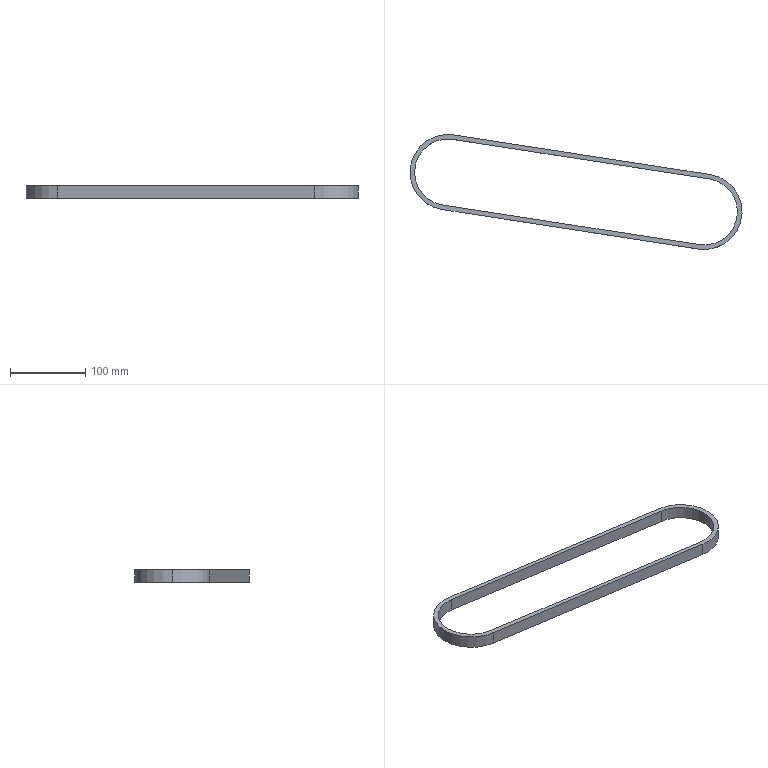Part | SolidWorks | features BeltProfileFeature 1, ExtruThin 1 | 1 solid | 12 faces | box 440 x 152.5 x 17 mm | volume 100304 mm3 | cylinder 6 | plane 6 | commonest cylinder face diameters 88 x3 100 x3
STEP:
#1=CARTESIAN_POINT('',(-44.,0.,8.5));
#2=VERTEX_POINT('',#1);
#3=CARTESIAN_POINT('',(6.715,43.485,8.5));
#4=VERTEX_POINT('',#3);
#5=CARTESIAN_POINT('',(0.,0.,8.5));
#6=DIRECTION('',(0.,0.,-1.));
#7=DIRECTION('',(-1.,0.,0.));
#8=AXIS2_PLACEMENT_3D('',#5,#6,#7);
#9=CIRCLE('',#8,44.);
#10=EDGE_CURVE('',#2,#4,#9,.T.);
#11=ORIENTED_EDGE('',*,*,#10,.F.);
#12=CARTESIAN_POINT('',(-44.,0.,-8.5));
#13=VERTEX_POINT('',#12);
#14=CARTESIAN_POINT('',(-44.,0.,8.5));
#15=DIRECTION('',(0.,0.,-1.));
#16=VECTOR('',#15,1000.);
#17=LINE('',#14,#16);
#18=EDGE_CURVE('',#2,#13,#17,.T.);
#19=ORIENTED_EDGE('',*,*,#18,.T.);
#20=CARTESIAN_POINT('',(6.715,43.485,-8.5));
#21=VERTEX_POINT('',#20);
#22=CARTESIAN_POINT('',(0.,0.,-8.5));
#23=DIRECTION('',(0.,0.,-1.));
#24=DIRECTION('',(-1.,0.,0.));
#25=AXIS2_PLACEMENT_3D('',#22,#23,#24);
#26=CIRCLE('',#25,44.);
#27=EDGE_CURVE('',#13,#21,#26,.T.);
#28=ORIENTED_EDGE('',*,*,#27,.T.);
#29=CARTESIAN_POINT('',(6.715,43.485,8.5));
#30=DIRECTION('',(0.,0.,-1.));
#31=VECTOR('',#30,1000.);
#32=LINE('',#29,#31);
#33=EDGE_CURVE('',#4,#21,#32,.T.);
#34=ORIENTED_EDGE('',*,*,#33,.F.);
#35=EDGE_LOOP('',(#11,#19,#28,#34));
#36=FACE_OUTER_BOUND('',#35,.T.);
#37=CARTESIAN_POINT('',(0.,0.,8.5));
#38=DIRECTION('',(0.,0.,-1.));
#39=DIRECTION('',(-1.,0.,0.));
#40=AXIS2_PLACEMENT_3D('',#37,#38,#39);
#41=CYLINDRICAL_SURFACE('',#40,44.);
#42=ADVANCED_FACE('',(#36),#41,.F.);
#43=CARTESIAN_POINT('',(-7.63,-49.414,8.5));
#44=VERTEX_POINT('',#43);
#45=CARTESIAN_POINT('',(-50.,0.,8.5));
#46=VERTEX_POINT('',#45);
#47=CARTESIAN_POINT('',(0.,0.,8.5));
#48=DIRECTION('',(0.,0.,-1.));
#49=DIRECTION('',(-1.,0.,0.));
#50=AXIS2_PLACEMENT_3D('',#47,#48,#49);
#51=CIRCLE('',#50,50.);
#52=EDGE_CURVE('',#44,#46,#51,.T.);
#53=ORIENTED_EDGE('',*,*,#52,.T.);
#54=CARTESIAN_POINT('',(-50.,0.,-8.5));
#55=VERTEX_POINT('',#54);
#56=CARTESIAN_POINT('',(-50.,0.,8.5));
#57=DIRECTION('',(0.,0.,-1.));
#58=VECTOR('',#57,1000.);
#59=LINE('',#56,#58);
#60=EDGE_CURVE('',#46,#55,#59,.T.);
#61=ORIENTED_EDGE('',*,*,#60,.T.);
#62=CARTESIAN_POINT('',(-7.63,-49.414,-8.5));
#63=VERTEX_POINT('',#62);
#64=CARTESIAN_POINT('',(0.,0.,-8.5));
#65=DIRECTION('',(0.,0.,-1.));
#66=DIRECTION('',(-1.,0.,0.));
#67=AXIS2_PLACEMENT_3D('',#64,#65,#66);
#68=CIRCLE('',#67,50.);
#69=EDGE_CURVE('',#63,#55,#68,.T.);
#70=ORIENTED_EDGE('',*,*,#69,.F.);
#71=CARTESIAN_POINT('',(-7.63,-49.414,8.5));
#72=DIRECTION('',(0.,0.,-1.));
#73=VECTOR('',#72,1000.);
#74=LINE('',#71,#73);
#75=EDGE_CURVE('',#44,#63,#74,.T.);
#76=ORIENTED_EDGE('',*,*,#75,.F.);
#77=EDGE_LOOP('',(#53,#61,#70,#76));
#78=FACE_OUTER_BOUND('',#77,.T.);
#79=CARTESIAN_POINT('',(0.,0.,8.5));
#80=DIRECTION('',(0.,0.,-1.));
#81=DIRECTION('',(-1.,0.,0.));
#82=AXIS2_PLACEMENT_3D('',#79,#80,#81);
#83=CYLINDRICAL_SURFACE('',#82,50.);
#84=ADVANCED_FACE('',(#78),#83,.T.);
#85=CARTESIAN_POINT('',(332.37,-101.914,-8.5));
#86=VERTEX_POINT('',#85);
#87=CARTESIAN_POINT('',(332.37,-101.914,-8.5));
#88=DIRECTION('',(-0.9883,0.1526,0.));
#89=VECTOR('',#88,1000.);
#90=LINE('',#87,#89);
#91=EDGE_CURVE('',#86,#63,#90,.T.);
#92=ORIENTED_EDGE('',*,*,#91,.F.);
#93=CARTESIAN_POINT('',(332.37,-101.914,8.5));
#94=VERTEX_POINT('',#93);
#95=CARTESIAN_POINT('',(332.37,-101.914,8.5));
#96=DIRECTION('',(0.,0.,-1.));
#97=VECTOR('',#96,1000.);
#98=LINE('',#95,#97);
#99=EDGE_CURVE('',#94,#86,#98,.T.);
#100=ORIENTED_EDGE('',*,*,#99,.F.);
#101=CARTESIAN_POINT('',(332.37,-101.914,8.5));
#102=DIRECTION('',(-0.9883,0.1526,0.));
#103=VECTOR('',#102,1000.);
#104=LINE('',#101,#103);
#105=EDGE_CURVE('',#94,#44,#104,.T.);
#106=ORIENTED_EDGE('',*,*,#105,.T.);
#107=ORIENTED_EDGE('',*,*,#75,.T.);
#108=EDGE_LOOP('',(#92,#100,#106,#107));
#109=FACE_OUTER_BOUND('',#108,.T.);
#110=CARTESIAN_POINT('',(332.37,-101.914,8.5));
#111=DIRECTION('',(-0.1526,-0.9883,0.));
#112=DIRECTION('',(0.9883,-0.1526,0.));
#113=AXIS2_PLACEMENT_3D('',#110,#111,#112);
#114=PLANE('',#113);
#115=ADVANCED_FACE('',(#109),#114,.T.);
#116=CARTESIAN_POINT('',(347.63,-3.086,-8.5));
#117=VERTEX_POINT('',#116);
#118=CARTESIAN_POINT('',(340.,-52.5,-8.5));
#119=DIRECTION('',(0.,0.,-1.));
#120=DIRECTION('',(-1.,0.,0.));
#121=AXIS2_PLACEMENT_3D('',#118,#119,#120);
#122=CIRCLE('',#121,50.);
#123=EDGE_CURVE('',#117,#86,#122,.T.);
#124=ORIENTED_EDGE('',*,*,#123,.F.);
#125=CARTESIAN_POINT('',(347.63,-3.086,8.5));
#126=VERTEX_POINT('',#125);
#127=CARTESIAN_POINT('',(347.63,-3.086,8.5));
#128=DIRECTION('',(0.,0.,-1.));
#129=VECTOR('',#128,1000.);
#130=LINE('',#127,#129);
#131=EDGE_CURVE('',#126,#117,#130,.T.);
#132=ORIENTED_EDGE('',*,*,#131,.F.);
#133=CARTESIAN_POINT('',(340.,-52.5,8.5));
#134=DIRECTION('',(0.,0.,-1.));
#135=DIRECTION('',(-1.,0.,0.));
#136=AXIS2_PLACEMENT_3D('',#133,#134,#135);
#137=CIRCLE('',#136,50.);
#138=EDGE_CURVE('',#126,#94,#137,.T.);
#139=ORIENTED_EDGE('',*,*,#138,.T.);
#140=ORIENTED_EDGE('',*,*,#99,.T.);
#141=EDGE_LOOP('',(#124,#132,#139,#140));
#142=FACE_OUTER_BOUND('',#141,.T.);
#143=CARTESIAN_POINT('',(340.,-52.5,8.5));
#144=DIRECTION('',(0.,0.,-1.));
#145=DIRECTION('',(-1.,0.,0.));
#146=AXIS2_PLACEMENT_3D('',#143,#144,#145);
#147=CYLINDRICAL_SURFACE('',#146,50.);
#148=ADVANCED_FACE('',(#142),#147,.T.);
#149=CARTESIAN_POINT('',(7.63,49.414,-8.5));
#150=VERTEX_POINT('',#149);
#151=CARTESIAN_POINT('',(7.63,49.414,-8.5));
#152=DIRECTION('',(0.9883,-0.1526,0.));
#153=VECTOR('',#152,1000.);
#154=LINE('',#151,#153);
#155=EDGE_CURVE('',#150,#117,#154,.T.);
#156=ORIENTED_EDGE('',*,*,#155,.F.);
#157=CARTESIAN_POINT('',(7.63,49.414,8.5));
#158=VERTEX_POINT('',#157);
#159=CARTESIAN_POINT('',(7.63,49.414,8.5));
#160=DIRECTION('',(0.,0.,-1.));
#161=VECTOR('',#160,1000.);
#162=LINE('',#159,#161);
#163=EDGE_CURVE('',#158,#150,#162,.T.);
#164=ORIENTED_EDGE('',*,*,#163,.F.);
#165=CARTESIAN_POINT('',(7.63,49.414,8.5));
#166=DIRECTION('',(0.9883,-0.1526,0.));
#167=VECTOR('',#166,1000.);
#168=LINE('',#165,#167);
#169=EDGE_CURVE('',#158,#126,#168,.T.);
#170=ORIENTED_EDGE('',*,*,#169,.T.);
#171=ORIENTED_EDGE('',*,*,#131,.T.);
#172=EDGE_LOOP('',(#156,#164,#170,#171));
#173=FACE_OUTER_BOUND('',#172,.T.);
#174=CARTESIAN_POINT('',(7.63,49.414,8.5));
#175=DIRECTION('',(0.1526,0.9883,0.));
#176=DIRECTION('',(-0.9883,0.1526,0.));
#177=AXIS2_PLACEMENT_3D('',#174,#175,#176);
#178=PLANE('',#177);
#179=ADVANCED_FACE('',(#173),#178,.T.);
#180=ORIENTED_EDGE('',*,*,#60,.F.);
#181=CARTESIAN_POINT('',(0.,0.,8.5));
#182=DIRECTION('',(0.,0.,-1.));
#183=DIRECTION('',(-1.,0.,0.));
#184=AXIS2_PLACEMENT_3D('',#181,#182,#183);
#185=CIRCLE('',#184,50.);
#186=EDGE_CURVE('',#46,#158,#185,.T.);
#187=ORIENTED_EDGE('',*,*,#186,.T.);
#188=ORIENTED_EDGE('',*,*,#163,.T.);
#189=CARTESIAN_POINT('',(0.,0.,-8.5));
#190=DIRECTION('',(0.,0.,-1.));
#191=DIRECTION('',(-1.,0.,0.));
#192=AXIS2_PLACEMENT_3D('',#189,#190,#191);
#193=CIRCLE('',#192,50.);
#194=EDGE_CURVE('',#55,#150,#193,.T.);
#195=ORIENTED_EDGE('',*,*,#194,.F.);
#196=EDGE_LOOP('',(#180,#187,#188,#195));
#197=FACE_OUTER_BOUND('',#196,.T.);
#198=CARTESIAN_POINT('',(0.,0.,8.5));
#199=DIRECTION('',(0.,0.,-1.));
#200=DIRECTION('',(-1.,0.,0.));
#201=AXIS2_PLACEMENT_3D('',#198,#199,#200);
#202=CYLINDRICAL_SURFACE('',#201,50.);
#203=ADVANCED_FACE('',(#197),#202,.T.);
#204=CARTESIAN_POINT('',(346.715,-9.015,8.5));
#205=VERTEX_POINT('',#204);
#206=CARTESIAN_POINT('',(333.285,-95.985,8.5));
#207=VERTEX_POINT('',#206);
#208=CARTESIAN_POINT('',(340.,-52.5,8.5));
#209=DIRECTION('',(0.,0.,-1.));
#210=DIRECTION('',(-1.,0.,0.));
#211=AXIS2_PLACEMENT_3D('',#208,#209,#210);
#212=CIRCLE('',#211,44.);
#213=EDGE_CURVE('',#205,#207,#212,.T.);
#214=ORIENTED_EDGE('',*,*,#213,.T.);
#215=CARTESIAN_POINT('',(-6.715,-43.485,8.5));
#216=VERTEX_POINT('',#215);
#217=CARTESIAN_POINT('',(-6.715,-43.485,8.5));
#218=DIRECTION('',(-0.9883,0.1526,0.));
#219=VECTOR('',#218,1000.);
#220=LINE('',#217,#219);
#221=EDGE_CURVE('',#207,#216,#220,.T.);
#222=ORIENTED_EDGE('',*,*,#221,.T.);
#223=CARTESIAN_POINT('',(0.,0.,8.5));
#224=DIRECTION('',(0.,0.,-1.));
#225=DIRECTION('',(-1.,0.,0.));
#226=AXIS2_PLACEMENT_3D('',#223,#224,#225);
#227=CIRCLE('',#226,44.);
#228=EDGE_CURVE('',#216,#2,#227,.T.);
#229=ORIENTED_EDGE('',*,*,#228,.T.);
#230=ORIENTED_EDGE('',*,*,#10,.T.);
#231=CARTESIAN_POINT('',(6.715,43.485,8.5));
#232=DIRECTION('',(0.9883,-0.1526,0.));
#233=VECTOR('',#232,1000.);
#234=LINE('',#231,#233);
#235=EDGE_CURVE('',#4,#205,#234,.T.);
#236=ORIENTED_EDGE('',*,*,#235,.T.);
#237=EDGE_LOOP('',(#214,#222,#229,#230,#236));
#238=FACE_BOUND('',#237,.T.);
#239=ORIENTED_EDGE('',*,*,#105,.F.);
#240=ORIENTED_EDGE('',*,*,#138,.F.);
#241=ORIENTED_EDGE('',*,*,#169,.F.);
#242=ORIENTED_EDGE('',*,*,#186,.F.);
#243=ORIENTED_EDGE('',*,*,#52,.F.);
#244=EDGE_LOOP('',(#239,#240,#241,#242,#243));
#245=FACE_OUTER_BOUND('',#244,.T.);
#246=CARTESIAN_POINT('',(0.,0.,8.5));
#247=DIRECTION('',(0.,0.,-1.));
#248=DIRECTION('',(-1.,0.,0.));
#249=AXIS2_PLACEMENT_3D('',#246,#247,#248);
#250=PLANE('',#249);
#251=ADVANCED_FACE('',(#238,#245),#250,.F.);
#252=CARTESIAN_POINT('',(333.285,-95.985,-8.5));
#253=VERTEX_POINT('',#252);
#254=CARTESIAN_POINT('',(-6.715,-43.485,-8.5));
#255=VERTEX_POINT('',#254);
#256=CARTESIAN_POINT('',(-6.715,-43.485,-8.5));
#257=DIRECTION('',(-0.9883,0.1526,0.));
#258=VECTOR('',#257,1000.);
#259=LINE('',#256,#258);
#260=EDGE_CURVE('',#253,#255,#259,.T.);
#261=ORIENTED_EDGE('',*,*,#260,.F.);
#262=CARTESIAN_POINT('',(346.715,-9.015,-8.5));
#263=VERTEX_POINT('',#262);
#264=CARTESIAN_POINT('',(340.,-52.5,-8.5));
#265=DIRECTION('',(0.,0.,-1.));
#266=DIRECTION('',(-1.,0.,0.));
#267=AXIS2_PLACEMENT_3D('',#264,#265,#266);
#268=CIRCLE('',#267,44.);
#269=EDGE_CURVE('',#263,#253,#268,.T.);
#270=ORIENTED_EDGE('',*,*,#269,.F.);
#271=CARTESIAN_POINT('',(6.715,43.485,-8.5));
#272=DIRECTION('',(0.9883,-0.1526,0.));
#273=VECTOR('',#272,1000.);
#274=LINE('',#271,#273);
#275=EDGE_CURVE('',#21,#263,#274,.T.);
#276=ORIENTED_EDGE('',*,*,#275,.F.);
#277=ORIENTED_EDGE('',*,*,#27,.F.);
#278=CARTESIAN_POINT('',(0.,0.,-8.5));
#279=DIRECTION('',(0.,0.,-1.));
#280=DIRECTION('',(-1.,0.,0.));
#281=AXIS2_PLACEMENT_3D('',#278,#279,#280);
#282=CIRCLE('',#281,44.);
#283=EDGE_CURVE('',#255,#13,#282,.T.);
#284=ORIENTED_EDGE('',*,*,#283,.F.);
#285=EDGE_LOOP('',(#261,#270,#276,#277,#284));
#286=FACE_BOUND('',#285,.T.);
#287=ORIENTED_EDGE('',*,*,#91,.T.);
#288=ORIENTED_EDGE('',*,*,#69,.T.);
#289=ORIENTED_EDGE('',*,*,#194,.T.);
#290=ORIENTED_EDGE('',*,*,#155,.T.);
#291=ORIENTED_EDGE('',*,*,#123,.T.);
#292=EDGE_LOOP('',(#287,#288,#289,#290,#291));
#293=FACE_OUTER_BOUND('',#292,.T.);
#294=CARTESIAN_POINT('',(0.,0.,-8.5));
#295=DIRECTION('',(0.,0.,-1.));
#296=DIRECTION('',(-1.,0.,0.));
#297=AXIS2_PLACEMENT_3D('',#294,#295,#296);
#298=PLANE('',#297);
#299=ADVANCED_FACE('',(#286,#293),#298,.T.);
#300=ORIENTED_EDGE('',*,*,#260,.T.);
#301=CARTESIAN_POINT('',(-6.715,-43.485,8.5));
#302=DIRECTION('',(0.,0.,-1.));
#303=VECTOR('',#302,1000.);
#304=LINE('',#301,#303);
#305=EDGE_CURVE('',#216,#255,#304,.T.);
#306=ORIENTED_EDGE('',*,*,#305,.F.);
#307=ORIENTED_EDGE('',*,*,#221,.F.);
#308=CARTESIAN_POINT('',(333.285,-95.985,8.5));
#309=DIRECTION('',(0.,0.,-1.));
#310=VECTOR('',#309,1000.);
#311=LINE('',#308,#310);
#312=EDGE_CURVE('',#207,#253,#311,.T.);
#313=ORIENTED_EDGE('',*,*,#312,.T.);
#314=EDGE_LOOP('',(#300,#306,#307,#313));
#315=FACE_OUTER_BOUND('',#314,.T.);
#316=CARTESIAN_POINT('',(-6.715,-43.485,8.5));
#317=DIRECTION('',(-0.1526,-0.9883,0.));
#318=DIRECTION('',(0.9883,-0.1526,0.));
#319=AXIS2_PLACEMENT_3D('',#316,#317,#318);
#320=PLANE('',#319);
#321=ADVANCED_FACE('',(#315),#320,.F.);
#322=ORIENTED_EDGE('',*,*,#269,.T.);
#323=ORIENTED_EDGE('',*,*,#312,.F.);
#324=ORIENTED_EDGE('',*,*,#213,.F.);
#325=CARTESIAN_POINT('',(346.715,-9.015,8.5));
#326=DIRECTION('',(0.,0.,-1.));
#327=VECTOR('',#326,1000.);
#328=LINE('',#325,#327);
#329=EDGE_CURVE('',#205,#263,#328,.T.);
#330=ORIENTED_EDGE('',*,*,#329,.T.);
#331=EDGE_LOOP('',(#322,#323,#324,#330));
#332=FACE_OUTER_BOUND('',#331,.T.);
#333=CARTESIAN_POINT('',(340.,-52.5,8.5));
#334=DIRECTION('',(0.,0.,-1.));
#335=DIRECTION('',(-1.,0.,0.));
#336=AXIS2_PLACEMENT_3D('',#333,#334,#335);
#337=CYLINDRICAL_SURFACE('',#336,44.);
#338=ADVANCED_FACE('',(#332),#337,.F.);
#339=ORIENTED_EDGE('',*,*,#275,.T.);
#340=ORIENTED_EDGE('',*,*,#329,.F.);
#341=ORIENTED_EDGE('',*,*,#235,.F.);
#342=ORIENTED_EDGE('',*,*,#33,.T.);
#343=EDGE_LOOP('',(#339,#340,#341,#342));
#344=FACE_OUTER_BOUND('',#343,.T.);
#345=CARTESIAN_POINT('',(6.715,43.485,8.5));
#346=DIRECTION('',(0.1526,0.9883,0.));
#347=DIRECTION('',(-0.9883,0.1526,0.));
#348=AXIS2_PLACEMENT_3D('',#345,#346,#347);
#349=PLANE('',#348);
#350=ADVANCED_FACE('',(#344),#349,.F.);
#351=ORIENTED_EDGE('',*,*,#18,.F.);
#352=ORIENTED_EDGE('',*,*,#228,.F.);
#353=ORIENTED_EDGE('',*,*,#305,.T.);
#354=ORIENTED_EDGE('',*,*,#283,.T.);
#355=EDGE_LOOP('',(#351,#352,#353,#354));
#356=FACE_OUTER_BOUND('',#355,.T.);
#357=CARTESIAN_POINT('',(0.,0.,8.5));
#358=DIRECTION('',(0.,0.,-1.));
#359=DIRECTION('',(-1.,0.,0.));
#360=AXIS2_PLACEMENT_3D('',#357,#358,#359);
#361=CYLINDRICAL_SURFACE('',#360,44.);
#362=ADVANCED_FACE('',(#356),#361,.F.);
#363=CLOSED_SHELL('',(#42,#84,#115,#148,#179,#203,#251,#299,#321,#338,#350,#362));
#364=MANIFOLD_SOLID_BREP('',#363);
#365=CARTESIAN_POINT('',(0.,0.,0.));
#366=DIRECTION('',(0.,0.,1.));
#367=DIRECTION('',(1.,0.,0.));
#368=AXIS2_PLACEMENT_3D('',#365,#366,#367);
#369=(LENGTH_UNIT()NAMED_UNIT(*)SI_UNIT(.MILLI.,.METRE.));
#370=UNCERTAINTY_MEASURE_WITH_UNIT(LENGTH_MEASURE(0.00001),#369,'','');
#371=(NAMED_UNIT(*)PLANE_ANGLE_UNIT()SI_UNIT($,.RADIAN.));
#372=(NAMED_UNIT(*)SI_UNIT($,.STERADIAN.)SOLID_ANGLE_UNIT());
#373=(GEOMETRIC_REPRESENTATION_CONTEXT(3)GLOBAL_UNCERTAINTY_ASSIGNED_CONTEXT((#370))GLOBAL_UNIT_ASSIGNED_CONTEXT((#369,#371,#372))REPRESENTATION_CONTEXT('',''));
#374=ADVANCED_BREP_SHAPE_REPRESENTATION('',(#364,#368),#373);